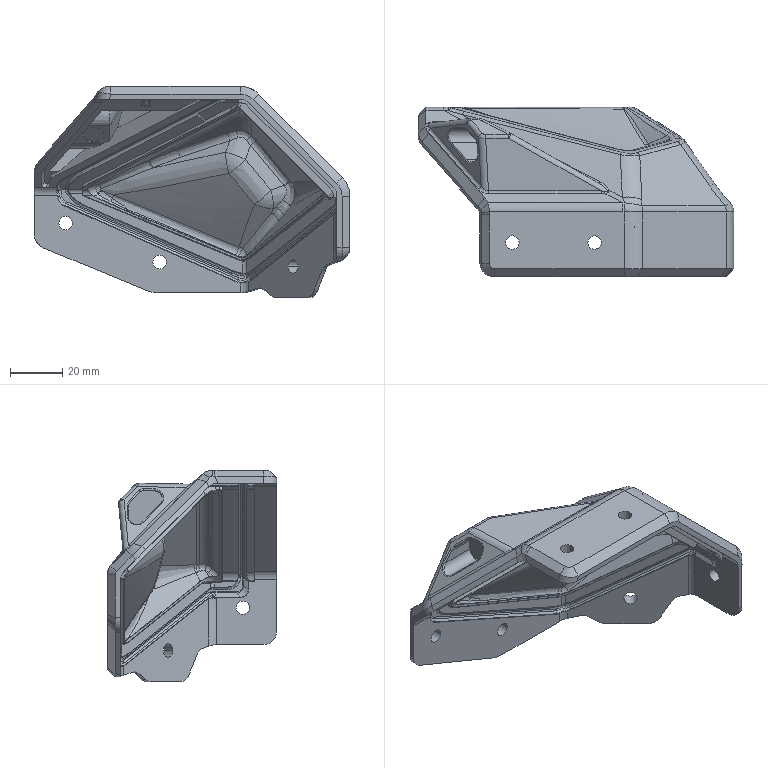Part | SolidWorks | features BaseBody 1 | 1 solid | 534 faces | box 121.207 x 65.033 x 81.159 mm | volume 62017 mm3 | spline 189 | plane 168 | cylinder 160 | sphere 6 | cone 6 | torus 5 | commonest cylinder face diameters 0.6 x16 0.4 x15 4 x15 5.2 x13 10 x13 8 x12